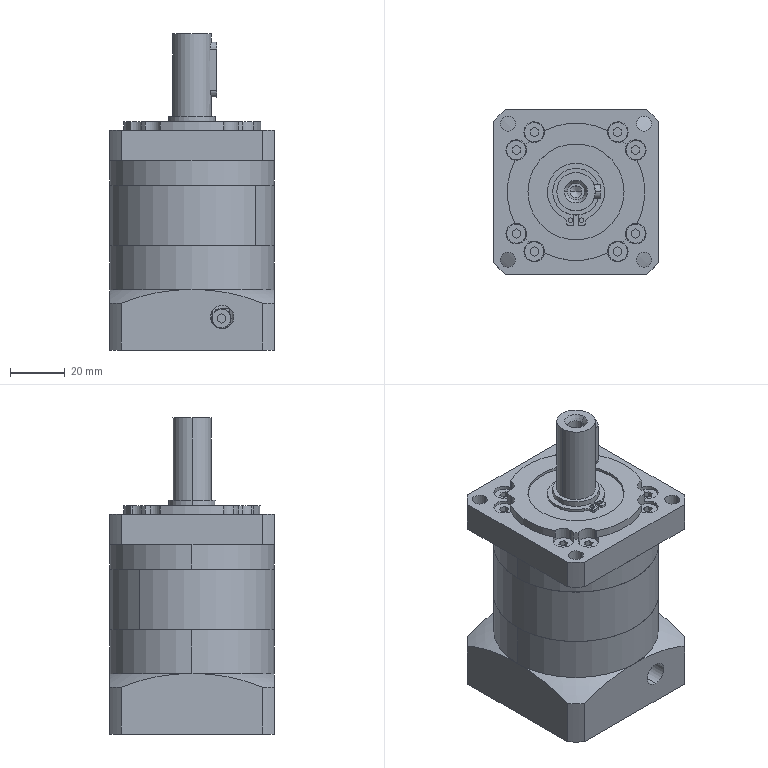Part | SolidWorks | features BaseBody 7 | 7 solids | 501 faces | box 60 x 60 x 115 mm | volume 222679 mm3 | cylinder 186 | plane 182 | spline 118 | cone 15 | commonest cylinder face diameters 7 x18 7.5 x17 5 x14 50 x14 20 x12 3.3 x10